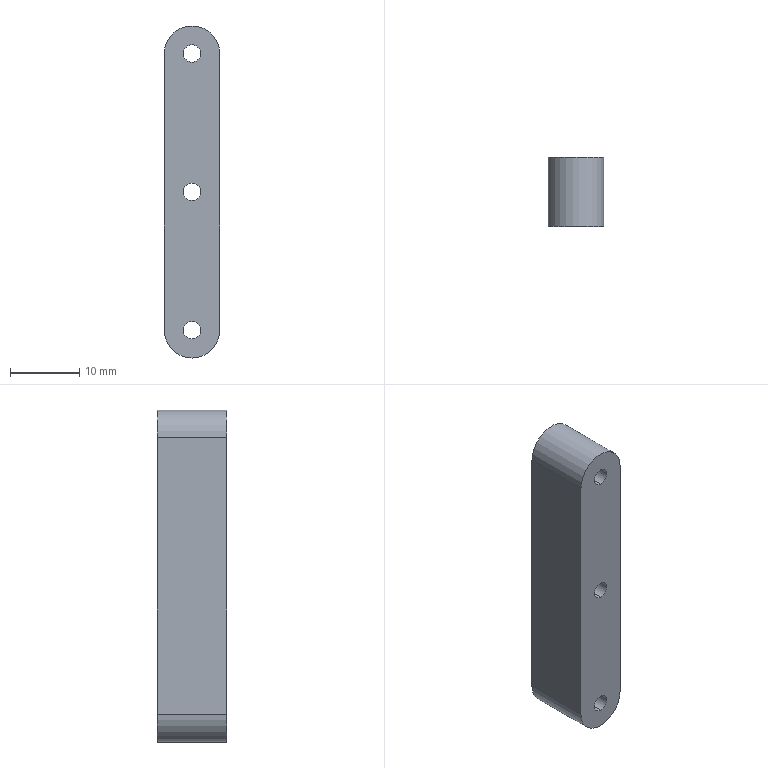Part | STEP file | 0246_209_Block | 1 solid | 13 faces | box 8 x 10 x 48 mm | volume 3555 mm3 | cylinder 9 | plane 4 | commonest cylinder face diameters 2.5 x6 8 x3
STEP:
#1=CARTESIAN_POINT('',(0.,0.,0.));
#2=DIRECTION('',(0.,0.,1.));
#3=DIRECTION('',(1.,0.,0.));
#4=AXIS2_PLACEMENT_3D('',#1,#2,#3);
#5=CARTESIAN_POINT('',(0.,0.,1.25));
#6=VERTEX_POINT('',#5);
#7=CARTESIAN_POINT('',(0.,10.,1.25));
#8=VERTEX_POINT('',#7);
#9=CARTESIAN_POINT('',(0.,10.,1.25));
#10=DIRECTION('',(0.,1.,0.));
#11=VECTOR('',#10,1.);
#12=LINE('',#9,#11);
#13=CARTESIAN_POINT('',(0.,10.,0.));
#14=DIRECTION('',(0.,1.,0.));
#15=DIRECTION('',(0.,0.,1.));
#16=AXIS2_PLACEMENT_3D('',#13,#14,#15);
#17=CYLINDRICAL_SURFACE('',#16,1.25);
#18=CARTESIAN_POINT('',(6.283,0.));
#19=DIRECTION('',(0.,1.));
#20=VECTOR('',#19,1.);
#21=LINE('',#18,#20);
#22=(GEOMETRIC_REPRESENTATION_CONTEXT(2)PARAMETRIC_REPRESENTATION_CONTEXT()REPRESENTATION_CONTEXT('',''));
#23=DEFINITIONAL_REPRESENTATION('',(#21),#22);
#24=PCURVE('',#17,#23);
#25=CARTESIAN_POINT('',(0.,10.,0.));
#26=DIRECTION('',(0.,1.,0.));
#27=DIRECTION('',(0.,0.,1.));
#28=AXIS2_PLACEMENT_3D('',#25,#26,#27);
#29=CYLINDRICAL_SURFACE('',#28,1.25);
#30=CARTESIAN_POINT('',(0.,0.));
#31=DIRECTION('',(0.,1.));
#32=VECTOR('',#31,1.);
#33=LINE('',#30,#32);
#34=(GEOMETRIC_REPRESENTATION_CONTEXT(2)PARAMETRIC_REPRESENTATION_CONTEXT()REPRESENTATION_CONTEXT('',''));
#35=DEFINITIONAL_REPRESENTATION('',(#33),#34);
#36=PCURVE('',#29,#35);
#37=SURFACE_CURVE('',#12,(#24,#36),.PCURVE_S1.);
#38=EDGE_CURVE('',#6,#8,#37,.T.);
#39=ORIENTED_EDGE('',*,*,#38,.T.);
#40=CARTESIAN_POINT('',(0.,10.,-1.25));
#41=VERTEX_POINT('',#40);
#42=CARTESIAN_POINT('',(0.,10.,0.));
#43=DIRECTION('',(0.,1.,0.));
#44=DIRECTION('',(0.,0.,1.));
#45=AXIS2_PLACEMENT_3D('',#42,#43,#44);
#46=CIRCLE('',#45,1.25);
#47=CARTESIAN_POINT('',(0.,0.));
#48=DIRECTION('',(1.,0.));
#49=VECTOR('',#48,1.);
#50=LINE('',#47,#49);
#51=(GEOMETRIC_REPRESENTATION_CONTEXT(2)PARAMETRIC_REPRESENTATION_CONTEXT()REPRESENTATION_CONTEXT('',''));
#52=DEFINITIONAL_REPRESENTATION('',(#50),#51);
#53=PCURVE('',#17,#52);
#54=CARTESIAN_POINT('',(0.,10.,0.));
#55=DIRECTION('',(0.,1.,0.));
#56=DIRECTION('',(0.,0.,1.));
#57=AXIS2_PLACEMENT_3D('',#54,#55,#56);
#58=PLANE('',#57);
#59=CARTESIAN_POINT('',(0.,0.));
#60=DIRECTION('',(1.,0.));
#61=AXIS2_PLACEMENT_2D('',#59,#60);
#62=CIRCLE('',#61,1.25);
#63=(GEOMETRIC_REPRESENTATION_CONTEXT(2)PARAMETRIC_REPRESENTATION_CONTEXT()REPRESENTATION_CONTEXT('',''));
#64=DEFINITIONAL_REPRESENTATION('',(#62),#63);
#65=PCURVE('',#58,#64);
#66=SURFACE_CURVE('',#46,(#53,#65),.PCURVE_S1.);
#67=EDGE_CURVE('',#41,#8,#66,.T.);
#68=ORIENTED_EDGE('',*,*,#67,.F.);
#69=CARTESIAN_POINT('',(0.,0.,-1.25));
#70=VERTEX_POINT('',#69);
#71=CARTESIAN_POINT('',(0.,10.,-1.25));
#72=DIRECTION('',(0.,1.,0.));
#73=VECTOR('',#72,1.);
#74=LINE('',#71,#73);
#75=CARTESIAN_POINT('',(3.142,0.));
#76=DIRECTION('',(0.,1.));
#77=VECTOR('',#76,1.);
#78=LINE('',#75,#77);
#79=(GEOMETRIC_REPRESENTATION_CONTEXT(2)PARAMETRIC_REPRESENTATION_CONTEXT()REPRESENTATION_CONTEXT('',''));
#80=DEFINITIONAL_REPRESENTATION('',(#78),#79);
#81=PCURVE('',#17,#80);
#82=CARTESIAN_POINT('',(3.142,0.));
#83=DIRECTION('',(0.,1.));
#84=VECTOR('',#83,1.);
#85=LINE('',#82,#84);
#86=(GEOMETRIC_REPRESENTATION_CONTEXT(2)PARAMETRIC_REPRESENTATION_CONTEXT()REPRESENTATION_CONTEXT('',''));
#87=DEFINITIONAL_REPRESENTATION('',(#85),#86);
#88=PCURVE('',#29,#87);
#89=SURFACE_CURVE('',#74,(#81,#88),.PCURVE_S1.);
#90=EDGE_CURVE('',#70,#41,#89,.T.);
#91=ORIENTED_EDGE('',*,*,#90,.F.);
#92=CARTESIAN_POINT('',(0.,0.,0.));
#93=DIRECTION('',(0.,1.,0.));
#94=DIRECTION('',(0.,0.,1.));
#95=AXIS2_PLACEMENT_3D('',#92,#93,#94);
#96=CIRCLE('',#95,1.25);
#97=CARTESIAN_POINT('',(0.,-10.));
#98=DIRECTION('',(1.,0.));
#99=VECTOR('',#98,1.);
#100=LINE('',#97,#99);
#101=(GEOMETRIC_REPRESENTATION_CONTEXT(2)PARAMETRIC_REPRESENTATION_CONTEXT()REPRESENTATION_CONTEXT('',''));
#102=DEFINITIONAL_REPRESENTATION('',(#100),#101);
#103=PCURVE('',#17,#102);
#104=CARTESIAN_POINT('',(0.,0.,0.));
#105=DIRECTION('',(0.,1.,0.));
#106=DIRECTION('',(0.,0.,1.));
#107=AXIS2_PLACEMENT_3D('',#104,#105,#106);
#108=PLANE('',#107);
#109=CARTESIAN_POINT('',(0.,0.));
#110=DIRECTION('',(1.,0.));
#111=AXIS2_PLACEMENT_2D('',#109,#110);
#112=CIRCLE('',#111,1.25);
#113=(GEOMETRIC_REPRESENTATION_CONTEXT(2)PARAMETRIC_REPRESENTATION_CONTEXT()REPRESENTATION_CONTEXT('',''));
#114=DEFINITIONAL_REPRESENTATION('',(#112),#113);
#115=PCURVE('',#108,#114);
#116=SURFACE_CURVE('',#96,(#103,#115),.PCURVE_S1.);
#117=EDGE_CURVE('',#70,#6,#116,.T.);
#118=ORIENTED_EDGE('',*,*,#117,.T.);
#119=EDGE_LOOP('',(#39,#68,#91,#118));
#120=FACE_BOUND('',#119,.F.);
#121=ADVANCED_FACE('',(#120),#17,.F.);
#122=CARTESIAN_POINT('',(0.,0.,-18.75));
#123=VERTEX_POINT('',#122);
#124=CARTESIAN_POINT('',(0.,10.,-18.75));
#125=VERTEX_POINT('',#124);
#126=CARTESIAN_POINT('',(0.,10.,-18.75));
#127=DIRECTION('',(0.,1.,0.));
#128=VECTOR('',#127,1.);
#129=LINE('',#126,#128);
#130=CARTESIAN_POINT('',(0.,10.,-20.));
#131=DIRECTION('',(0.,1.,0.));
#132=DIRECTION('',(0.,0.,1.));
#133=AXIS2_PLACEMENT_3D('',#130,#131,#132);
#134=CYLINDRICAL_SURFACE('',#133,1.25);
#135=CARTESIAN_POINT('',(6.283,0.));
#136=DIRECTION('',(0.,1.));
#137=VECTOR('',#136,1.);
#138=LINE('',#135,#137);
#139=(GEOMETRIC_REPRESENTATION_CONTEXT(2)PARAMETRIC_REPRESENTATION_CONTEXT()REPRESENTATION_CONTEXT('',''));
#140=DEFINITIONAL_REPRESENTATION('',(#138),#139);
#141=PCURVE('',#134,#140);
#142=CARTESIAN_POINT('',(0.,10.,-20.));
#143=DIRECTION('',(0.,1.,0.));
#144=DIRECTION('',(0.,0.,1.));
#145=AXIS2_PLACEMENT_3D('',#142,#143,#144);
#146=CYLINDRICAL_SURFACE('',#145,1.25);
#147=CARTESIAN_POINT('',(0.,0.));
#148=DIRECTION('',(0.,1.));
#149=VECTOR('',#148,1.);
#150=LINE('',#147,#149);
#151=(GEOMETRIC_REPRESENTATION_CONTEXT(2)PARAMETRIC_REPRESENTATION_CONTEXT()REPRESENTATION_CONTEXT('',''));
#152=DEFINITIONAL_REPRESENTATION('',(#150),#151);
#153=PCURVE('',#146,#152);
#154=SURFACE_CURVE('',#129,(#141,#153),.PCURVE_S1.);
#155=EDGE_CURVE('',#123,#125,#154,.T.);
#156=ORIENTED_EDGE('',*,*,#155,.T.);
#157=CARTESIAN_POINT('',(0.,10.,-21.25));
#158=VERTEX_POINT('',#157);
#159=CARTESIAN_POINT('',(0.,10.,-20.));
#160=DIRECTION('',(0.,1.,0.));
#161=DIRECTION('',(0.,0.,1.));
#162=AXIS2_PLACEMENT_3D('',#159,#160,#161);
#163=CIRCLE('',#162,1.25);
#164=CARTESIAN_POINT('',(0.,0.));
#165=DIRECTION('',(1.,0.));
#166=VECTOR('',#165,1.);
#167=LINE('',#164,#166);
#168=(GEOMETRIC_REPRESENTATION_CONTEXT(2)PARAMETRIC_REPRESENTATION_CONTEXT()REPRESENTATION_CONTEXT('',''));
#169=DEFINITIONAL_REPRESENTATION('',(#167),#168);
#170=PCURVE('',#134,#169);
#171=CARTESIAN_POINT('',(-20.,0.));
#172=DIRECTION('',(1.,0.));
#173=AXIS2_PLACEMENT_2D('',#171,#172);
#174=CIRCLE('',#173,1.25);
#175=(GEOMETRIC_REPRESENTATION_CONTEXT(2)PARAMETRIC_REPRESENTATION_CONTEXT()REPRESENTATION_CONTEXT('',''));
#176=DEFINITIONAL_REPRESENTATION('',(#174),#175);
#177=PCURVE('',#58,#176);
#178=SURFACE_CURVE('',#163,(#170,#177),.PCURVE_S1.);
#179=EDGE_CURVE('',#158,#125,#178,.T.);
#180=ORIENTED_EDGE('',*,*,#179,.F.);
#181=CARTESIAN_POINT('',(0.,0.,-21.25));
#182=VERTEX_POINT('',#181);
#183=CARTESIAN_POINT('',(0.,10.,-21.25));
#184=DIRECTION('',(0.,1.,0.));
#185=VECTOR('',#184,1.);
#186=LINE('',#183,#185);
#187=CARTESIAN_POINT('',(3.142,0.));
#188=DIRECTION('',(0.,1.));
#189=VECTOR('',#188,1.);
#190=LINE('',#187,#189);
#191=(GEOMETRIC_REPRESENTATION_CONTEXT(2)PARAMETRIC_REPRESENTATION_CONTEXT()REPRESENTATION_CONTEXT('',''));
#192=DEFINITIONAL_REPRESENTATION('',(#190),#191);
#193=PCURVE('',#134,#192);
#194=CARTESIAN_POINT('',(3.142,0.));
#195=DIRECTION('',(0.,1.));
#196=VECTOR('',#195,1.);
#197=LINE('',#194,#196);
#198=(GEOMETRIC_REPRESENTATION_CONTEXT(2)PARAMETRIC_REPRESENTATION_CONTEXT()REPRESENTATION_CONTEXT('',''));
#199=DEFINITIONAL_REPRESENTATION('',(#197),#198);
#200=PCURVE('',#146,#199);
#201=SURFACE_CURVE('',#186,(#193,#200),.PCURVE_S1.);
#202=EDGE_CURVE('',#182,#158,#201,.T.);
#203=ORIENTED_EDGE('',*,*,#202,.F.);
#204=CARTESIAN_POINT('',(0.,0.,-20.));
#205=DIRECTION('',(0.,1.,0.));
#206=DIRECTION('',(0.,0.,1.));
#207=AXIS2_PLACEMENT_3D('',#204,#205,#206);
#208=CIRCLE('',#207,1.25);
#209=CARTESIAN_POINT('',(0.,-10.));
#210=DIRECTION('',(1.,0.));
#211=VECTOR('',#210,1.);
#212=LINE('',#209,#211);
#213=(GEOMETRIC_REPRESENTATION_CONTEXT(2)PARAMETRIC_REPRESENTATION_CONTEXT()REPRESENTATION_CONTEXT('',''));
#214=DEFINITIONAL_REPRESENTATION('',(#212),#213);
#215=PCURVE('',#134,#214);
#216=CARTESIAN_POINT('',(-20.,0.));
#217=DIRECTION('',(1.,0.));
#218=AXIS2_PLACEMENT_2D('',#216,#217);
#219=CIRCLE('',#218,1.25);
#220=(GEOMETRIC_REPRESENTATION_CONTEXT(2)PARAMETRIC_REPRESENTATION_CONTEXT()REPRESENTATION_CONTEXT('',''));
#221=DEFINITIONAL_REPRESENTATION('',(#219),#220);
#222=PCURVE('',#108,#221);
#223=SURFACE_CURVE('',#208,(#215,#222),.PCURVE_S1.);
#224=EDGE_CURVE('',#182,#123,#223,.T.);
#225=ORIENTED_EDGE('',*,*,#224,.T.);
#226=EDGE_LOOP('',(#156,#180,#203,#225));
#227=FACE_BOUND('',#226,.F.);
#228=ADVANCED_FACE('',(#227),#134,.F.);
#229=CARTESIAN_POINT('',(0.,0.,-38.75));
#230=VERTEX_POINT('',#229);
#231=CARTESIAN_POINT('',(0.,10.,-38.75));
#232=VERTEX_POINT('',#231);
#233=CARTESIAN_POINT('',(0.,10.,-38.75));
#234=DIRECTION('',(0.,1.,0.));
#235=VECTOR('',#234,1.);
#236=LINE('',#233,#235);
#237=CARTESIAN_POINT('',(0.,10.,-40.));
#238=DIRECTION('',(0.,1.,0.));
#239=DIRECTION('',(0.,0.,1.));
#240=AXIS2_PLACEMENT_3D('',#237,#238,#239);
#241=CYLINDRICAL_SURFACE('',#240,1.25);
#242=CARTESIAN_POINT('',(6.283,0.));
#243=DIRECTION('',(0.,1.));
#244=VECTOR('',#243,1.);
#245=LINE('',#242,#244);
#246=(GEOMETRIC_REPRESENTATION_CONTEXT(2)PARAMETRIC_REPRESENTATION_CONTEXT()REPRESENTATION_CONTEXT('',''));
#247=DEFINITIONAL_REPRESENTATION('',(#245),#246);
#248=PCURVE('',#241,#247);
#249=CARTESIAN_POINT('',(0.,10.,-40.));
#250=DIRECTION('',(0.,1.,0.));
#251=DIRECTION('',(0.,0.,1.));
#252=AXIS2_PLACEMENT_3D('',#249,#250,#251);
#253=CYLINDRICAL_SURFACE('',#252,1.25);
#254=CARTESIAN_POINT('',(0.,0.));
#255=DIRECTION('',(0.,1.));
#256=VECTOR('',#255,1.);
#257=LINE('',#254,#256);
#258=(GEOMETRIC_REPRESENTATION_CONTEXT(2)PARAMETRIC_REPRESENTATION_CONTEXT()REPRESENTATION_CONTEXT('',''));
#259=DEFINITIONAL_REPRESENTATION('',(#257),#258);
#260=PCURVE('',#253,#259);
#261=SURFACE_CURVE('',#236,(#248,#260),.PCURVE_S1.);
#262=EDGE_CURVE('',#230,#232,#261,.T.);
#263=ORIENTED_EDGE('',*,*,#262,.T.);
#264=CARTESIAN_POINT('',(0.,10.,-41.25));
#265=VERTEX_POINT('',#264);
#266=CARTESIAN_POINT('',(0.,10.,-40.));
#267=DIRECTION('',(0.,1.,0.));
#268=DIRECTION('',(0.,0.,1.));
#269=AXIS2_PLACEMENT_3D('',#266,#267,#268);
#270=CIRCLE('',#269,1.25);
#271=CARTESIAN_POINT('',(0.,0.));
#272=DIRECTION('',(1.,0.));
#273=VECTOR('',#272,1.);
#274=LINE('',#271,#273);
#275=(GEOMETRIC_REPRESENTATION_CONTEXT(2)PARAMETRIC_REPRESENTATION_CONTEXT()REPRESENTATION_CONTEXT('',''));
#276=DEFINITIONAL_REPRESENTATION('',(#274),#275);
#277=PCURVE('',#241,#276);
#278=CARTESIAN_POINT('',(-40.,0.));
#279=DIRECTION('',(1.,0.));
#280=AXIS2_PLACEMENT_2D('',#278,#279);
#281=CIRCLE('',#280,1.25);
#282=(GEOMETRIC_REPRESENTATION_CONTEXT(2)PARAMETRIC_REPRESENTATION_CONTEXT()REPRESENTATION_CONTEXT('',''));
#283=DEFINITIONAL_REPRESENTATION('',(#281),#282);
#284=PCURVE('',#58,#283);
#285=SURFACE_CURVE('',#270,(#277,#284),.PCURVE_S1.);
#286=EDGE_CURVE('',#265,#232,#285,.T.);
#287=ORIENTED_EDGE('',*,*,#286,.F.);
#288=CARTESIAN_POINT('',(0.,0.,-41.25));
#289=VERTEX_POINT('',#288);
#290=CARTESIAN_POINT('',(0.,10.,-41.25));
#291=DIRECTION('',(0.,1.,0.));
#292=VECTOR('',#291,1.);
#293=LINE('',#290,#292);
#294=CARTESIAN_POINT('',(3.142,0.));
#295=DIRECTION('',(0.,1.));
#296=VECTOR('',#295,1.);
#297=LINE('',#294,#296);
#298=(GEOMETRIC_REPRESENTATION_CONTEXT(2)PARAMETRIC_REPRESENTATION_CONTEXT()REPRESENTATION_CONTEXT('',''));
#299=DEFINITIONAL_REPRESENTATION('',(#297),#298);
#300=PCURVE('',#241,#299);
#301=CARTESIAN_POINT('',(3.142,0.));
#302=DIRECTION('',(0.,1.));
#303=VECTOR('',#302,1.);
#304=LINE('',#301,#303);
#305=(GEOMETRIC_REPRESENTATION_CONTEXT(2)PARAMETRIC_REPRESENTATION_CONTEXT()REPRESENTATION_CONTEXT('',''));
#306=DEFINITIONAL_REPRESENTATION('',(#304),#305);
#307=PCURVE('',#253,#306);
#308=SURFACE_CURVE('',#293,(#300,#307),.PCURVE_S1.);
#309=EDGE_CURVE('',#289,#265,#308,.T.);
#310=ORIENTED_EDGE('',*,*,#309,.F.);
#311=CARTESIAN_POINT('',(0.,0.,-40.));
#312=DIRECTION('',(0.,1.,0.));
#313=DIRECTION('',(0.,0.,1.));
#314=AXIS2_PLACEMENT_3D('',#311,#312,#313);
#315=CIRCLE('',#314,1.25);
#316=CARTESIAN_POINT('',(0.,-10.));
#317=DIRECTION('',(1.,0.));
#318=VECTOR('',#317,1.);
#319=LINE('',#316,#318);
#320=(GEOMETRIC_REPRESENTATION_CONTEXT(2)PARAMETRIC_REPRESENTATION_CONTEXT()REPRESENTATION_CONTEXT('',''));
#321=DEFINITIONAL_REPRESENTATION('',(#319),#320);
#322=PCURVE('',#241,#321);
#323=CARTESIAN_POINT('',(-40.,0.));
#324=DIRECTION('',(1.,0.));
#325=AXIS2_PLACEMENT_2D('',#323,#324);
#326=CIRCLE('',#325,1.25);
#327=(GEOMETRIC_REPRESENTATION_CONTEXT(2)PARAMETRIC_REPRESENTATION_CONTEXT()REPRESENTATION_CONTEXT('',''));
#328=DEFINITIONAL_REPRESENTATION('',(#326),#327);
#329=PCURVE('',#108,#328);
#330=SURFACE_CURVE('',#315,(#322,#329),.PCURVE_S1.);
#331=EDGE_CURVE('',#289,#230,#330,.T.);
#332=ORIENTED_EDGE('',*,*,#331,.T.);
#333=EDGE_LOOP('',(#263,#287,#310,#332));
#334=FACE_BOUND('',#333,.F.);
#335=ADVANCED_FACE('',(#334),#241,.F.);
#336=CARTESIAN_POINT('',(0.,10.,-44.));
#337=VERTEX_POINT('',#336);
#338=CARTESIAN_POINT('',(-4.,10.,-40.));
#339=VERTEX_POINT('',#338);
#340=CARTESIAN_POINT('',(0.,10.,-40.));
#341=DIRECTION('',(0.,1.,0.));
#342=DIRECTION('',(0.,0.,1.));
#343=AXIS2_PLACEMENT_3D('',#340,#341,#342);
#344=CIRCLE('',#343,4.);
#345=CARTESIAN_POINT('',(0.,10.,-40.));
#346=DIRECTION('',(0.,-1.,0.));
#347=DIRECTION('',(0.,0.,-1.));
#348=AXIS2_PLACEMENT_3D('',#345,#346,#347);
#349=CYLINDRICAL_SURFACE('',#348,4.);
#350=CARTESIAN_POINT('',(9.425,0.));
#351=DIRECTION('',(-1.,0.));
#352=VECTOR('',#351,1.);
#353=LINE('',#350,#352);
#354=(GEOMETRIC_REPRESENTATION_CONTEXT(2)PARAMETRIC_REPRESENTATION_CONTEXT()REPRESENTATION_CONTEXT('',''));
#355=DEFINITIONAL_REPRESENTATION('',(#353),#354);
#356=PCURVE('',#349,#355);
#357=CARTESIAN_POINT('',(-40.,0.));
#358=DIRECTION('',(1.,0.));
#359=AXIS2_PLACEMENT_2D('',#357,#358);
#360=CIRCLE('',#359,4.);
#361=(GEOMETRIC_REPRESENTATION_CONTEXT(2)PARAMETRIC_REPRESENTATION_CONTEXT()REPRESENTATION_CONTEXT('',''));
#362=DEFINITIONAL_REPRESENTATION('',(#360),#361);
#363=PCURVE('',#58,#362);
#364=SURFACE_CURVE('',#344,(#356,#363),.PCURVE_S1.);
#365=EDGE_CURVE('',#337,#339,#364,.T.);
#366=ORIENTED_EDGE('',*,*,#365,.F.);
#367=CARTESIAN_POINT('',(0.,0.,-44.));
#368=VERTEX_POINT('',#367);
#369=CARTESIAN_POINT('',(0.,10.,-44.));
#370=DIRECTION('',(0.,-1.,0.));
#371=VECTOR('',#370,1.);
#372=LINE('',#369,#371);
#373=CARTESIAN_POINT('',(6.283,0.));
#374=DIRECTION('',(0.,1.));
#375=VECTOR('',#374,1.);
#376=LINE('',#373,#375);
#377=(GEOMETRIC_REPRESENTATION_CONTEXT(2)PARAMETRIC_REPRESENTATION_CONTEXT()REPRESENTATION_CONTEXT('',''));
#378=DEFINITIONAL_REPRESENTATION('',(#376),#377);
#379=PCURVE('',#349,#378);
#380=CARTESIAN_POINT('',(0.,10.,-40.));
#381=DIRECTION('',(0.,-1.,0.));
#382=DIRECTION('',(0.,0.,-1.));
#383=AXIS2_PLACEMENT_3D('',#380,#381,#382);
#384=CYLINDRICAL_SURFACE('',#383,4.);
#385=CARTESIAN_POINT('',(0.,0.));
#386=DIRECTION('',(0.,1.));
#387=VECTOR('',#386,1.);
#388=LINE('',#385,#387);
#389=(GEOMETRIC_REPRESENTATION_CONTEXT(2)PARAMETRIC_REPRESENTATION_CONTEXT()REPRESENTATION_CONTEXT('',''));
#390=DEFINITIONAL_REPRESENTATION('',(#388),#389);
#391=PCURVE('',#384,#390);
#392=SURFACE_CURVE('',#372,(#379,#391),.PCURVE_S1.);
#393=EDGE_CURVE('',#337,#368,#392,.T.);
#394=ORIENTED_EDGE('',*,*,#393,.T.);
#395=CARTESIAN_POINT('',(-4.,0.,-40.));
#396=VERTEX_POINT('',#395);
#397=CARTESIAN_POINT('',(0.,0.,-40.));
#398=DIRECTION('',(0.,1.,0.));
#399=DIRECTION('',(0.,0.,1.));
#400=AXIS2_PLACEMENT_3D('',#397,#398,#399);
#401=CIRCLE('',#400,4.);
#402=CARTESIAN_POINT('',(9.425,10.));
#403=DIRECTION('',(-1.,0.));
#404=VECTOR('',#403,1.);
#405=LINE('',#402,#404);
#406=(GEOMETRIC_REPRESENTATION_CONTEXT(2)PARAMETRIC_REPRESENTATION_CONTEXT()REPRESENTATION_CONTEXT('',''));
#407=DEFINITIONAL_REPRESENTATION('',(#405),#406);
#408=PCURVE('',#349,#407);
#409=CARTESIAN_POINT('',(-40.,0.));
#410=DIRECTION('',(1.,0.));
#411=AXIS2_PLACEMENT_2D('',#409,#410);
#412=CIRCLE('',#411,4.);
#413=(GEOMETRIC_REPRESENTATION_CONTEXT(2)PARAMETRIC_REPRESENTATION_CONTEXT()REPRESENTATION_CONTEXT('',''));
#414=DEFINITIONAL_REPRESENTATION('',(#412),#413);
#415=PCURVE('',#108,#414);
#416=SURFACE_CURVE('',#401,(#408,#415),.PCURVE_S1.);
#417=EDGE_CURVE('',#368,#396,#416,.T.);
#418=ORIENTED_EDGE('',*,*,#417,.T.);
#419=CARTESIAN_POINT('',(-4.,10.,-40.));
#420=DIRECTION('',(0.,-1.,0.));
#421=VECTOR('',#420,1.);
#422=LINE('',#419,#421);
#423=CARTESIAN_POINT('',(4.712,0.));
#424=DIRECTION('',(0.,1.));
#425=VECTOR('',#424,1.);
#426=LINE('',#423,#425);
#427=(GEOMETRIC_REPRESENTATION_CONTEXT(2)PARAMETRIC_REPRESENTATION_CONTEXT()REPRESENTATION_CONTEXT('',''));
#428=DEFINITIONAL_REPRESENTATION('',(#426),#427);
#429=PCURVE('',#349,#428);
#430=CARTESIAN_POINT('',(-4.,10.,0.));
#431=DIRECTION('',(1.,0.,0.));
#432=DIRECTION('',(0.,0.,-1.));
#433=AXIS2_PLACEMENT_3D('',#430,#431,#432);
#434=PLANE('',#433);
#435=CARTESIAN_POINT('',(40.,0.));
#436=DIRECTION('',(0.,-1.));
#437=VECTOR('',#436,1.);
#438=LINE('',#435,#437);
#439=(GEOMETRIC_REPRESENTATION_CONTEXT(2)PARAMETRIC_REPRESENTATION_CONTEXT()REPRESENTATION_CONTEXT('',''));
#440=DEFINITIONAL_REPRESENTATION('',(#438),#439);
#441=PCURVE('',#434,#440);
#442=SURFACE_CURVE('',#422,(#429,#441),.PCURVE_S1.);
#443=EDGE_CURVE('',#339,#396,#442,.T.);
#444=ORIENTED_EDGE('',*,*,#443,.F.);
#445=EDGE_LOOP('',(#366,#394,#418,#444));
#446=FACE_BOUND('',#445,.T.);
#447=ADVANCED_FACE('',(#446),#349,.T.);
#448=CARTESIAN_POINT('',(-4.,0.,0.));
#449=VERTEX_POINT('',#448);
#450=CARTESIAN_POINT('',(4.,0.,0.));
#451=VERTEX_POINT('',#450);
#452=CARTESIAN_POINT('',(0.,0.,0.));
#453=DIRECTION('',(0.,1.,0.));
#454=DIRECTION('',(0.,0.,1.));
#455=AXIS2_PLACEMENT_3D('',#452,#453,#454);
#456=CIRCLE('',#455,4.);
#457=CARTESIAN_POINT('',(0.,10.,0.));
#458=DIRECTION('',(0.,-1.,0.));
#459=DIRECTION('',(0.,0.,-1.));
#460=AXIS2_PLACEMENT_3D('',#457,#458,#459);
#461=CYLINDRICAL_SURFACE('',#460,4.);
#462=CARTESIAN_POINT('',(9.425,10.));
#463=DIRECTION('',(-1.,0.));
#464=VECTOR('',#463,1.);
#465=LINE('',#462,#464);
#466=(GEOMETRIC_REPRESENTATION_CONTEXT(2)PARAMETRIC_REPRESENTATION_CONTEXT()REPRESENTATION_CONTEXT('',''));
#467=DEFINITIONAL_REPRESENTATION('',(#465),#466);
#468=PCURVE('',#461,#467);
#469=CARTESIAN_POINT('',(0.,0.));
#470=DIRECTION('',(1.,0.));
#471=AXIS2_PLACEMENT_2D('',#469,#470);
#472=CIRCLE('',#471,4.);
#473=(GEOMETRIC_REPRESENTATION_CONTEXT(2)PARAMETRIC_REPRESENTATION_CONTEXT()REPRESENTATION_CONTEXT('',''));
#474=DEFINITIONAL_REPRESENTATION('',(#472),#473);
#475=PCURVE('',#108,#474);
#476=SURFACE_CURVE('',#456,(#468,#475),.PCURVE_S1.);
#477=EDGE_CURVE('',#449,#451,#476,.T.);
#478=ORIENTED_EDGE('',*,*,#477,.T.);
#479=CARTESIAN_POINT('',(4.,10.,0.));
#480=VERTEX_POINT('',#479);
#481=CARTESIAN_POINT('',(4.,10.,0.));
#482=DIRECTION('',(0.,-1.,0.));
#483=VECTOR('',#482,1.);
#484=LINE('',#481,#483);
#485=CARTESIAN_POINT('',(1.571,0.));
#486=DIRECTION('',(0.,1.));
#487=VECTOR('',#486,1.);
#488=LINE('',#485,#487);
#489=(GEOMETRIC_REPRESENTATION_CONTEXT(2)PARAMETRIC_REPRESENTATION_CONTEXT()REPRESENTATION_CONTEXT('',''));
#490=DEFINITIONAL_REPRESENTATION('',(#488),#489);
#491=PCURVE('',#461,#490);
#492=CARTESIAN_POINT('',(4.,10.,0.));
#493=DIRECTION('',(-1.,0.,0.));
#494=DIRECTION('',(0.,0.,1.));
#495=AXIS2_PLACEMENT_3D('',#492,#493,#494);
#496=PLANE('',#495);
#497=CARTESIAN_POINT('',(0.,0.));
#498=DIRECTION('',(0.,-1.));
#499=VECTOR('',#498,1.);
#500=LINE('',#497,#499);
#501=(GEOMETRIC_REPRESENTATION_CONTEXT(2)PARAMETRIC_REPRESENTATION_CONTEXT()REPRESENTATION_CONTEXT('',''));
#502=DEFINITIONAL_REPRESENTATION('',(#500),#501);
#503=PCURVE('',#496,#502);
#504=SURFACE_CURVE('',#484,(#491,#503),.PCURVE_S1.);
#505=EDGE_CURVE('',#480,#451,#504,.T.);
#506=ORIENTED_EDGE('',*,*,#505,.F.);
#507=CARTESIAN_POINT('',(-4.,10.,0.));
#508=VERTEX_POINT('',#507);
#509=CARTESIAN_POINT('',(0.,10.,0.));
#510=DIRECTION('',(0.,1.,0.));
#511=DIRECTION('',(0.,0.,1.));
#512=AXIS2_PLACEMENT_3D('',#509,#510,#511);
#513=CIRCLE('',#512,4.);
#514=CARTESIAN_POINT('',(9.425,0.));
#515=DIRECTION('',(-1.,0.));
#516=VECTOR('',#515,1.);
#517=LINE('',#514,#516);
#518=(GEOMETRIC_REPRESENTATION_CONTEXT(2)PARAMETRIC_REPRESENTATION_CONTEXT()REPRESENTATION_CONTEXT('',''));
#519=DEFINITIONAL_REPRESENTATION('',(#517),#518);
#520=PCURVE('',#461,#519);
#521=CARTESIAN_POINT('',(0.,0.));
#522=DIRECTION('',(1.,0.));
#523=AXIS2_PLACEMENT_2D('',#521,#522);
#524=CIRCLE('',#523,4.);
#525=(GEOMETRIC_REPRESENTATION_CONTEXT(2)PARAMETRIC_REPRESENTATION_CONTEXT()REPRESENTATION_CONTEXT('',''));
#526=DEFINITIONAL_REPRESENTATION('',(#524),#525);
#527=PCURVE('',#58,#526);
#528=SURFACE_CURVE('',#513,(#520,#527),.PCURVE_S1.);
#529=EDGE_CURVE('',#508,#480,#528,.T.);
#530=ORIENTED_EDGE('',*,*,#529,.F.);
#531=CARTESIAN_POINT('',(-4.,10.,0.));
#532=DIRECTION('',(0.,-1.,0.));
#533=VECTOR('',#532,1.);
#534=LINE('',#531,#533);
#535=CARTESIAN_POINT('',(4.712,0.));
#536=DIRECTION('',(0.,1.));
#537=VECTOR('',#536,1.);
#538=LINE('',#535,#537);
#539=(GEOMETRIC_REPRESENTATION_CONTEXT(2)PARAMETRIC_REPRESENTATION_CONTEXT()REPRESENTATION_CONTEXT('',''));
#540=DEFINITIONAL_REPRESENTATION('',(#538),#539);
#541=PCURVE('',#461,#540);
#542=CARTESIAN_POINT('',(0.,0.));
#543=DIRECTION('',(0.,-1.));
#544=VECTOR('',#543,1.);
#545=LINE('',#542,#544);
#546=(GEOMETRIC_REPRESENTATION_CONTEXT(2)PARAMETRIC_REPRESENTATION_CONTEXT()REPRESENTATION_CONTEXT('',''));
#547=DEFINITIONAL_REPRESENTATION('',(#545),#546);
#548=PCURVE('',#434,#547);
#549=SURFACE_CURVE('',#534,(#541,#548),.PCURVE_S1.);
#550=EDGE_CURVE('',#508,#449,#549,.T.);
#551=ORIENTED_EDGE('',*,*,#550,.T.);
#552=EDGE_LOOP('',(#478,#506,#530,#551));
#553=FACE_BOUND('',#552,.T.);
#554=ADVANCED_FACE('',(#553),#461,.T.);
#555=CARTESIAN_POINT('',(4.,0.,-40.));
#556=VERTEX_POINT('',#555);
#557=CARTESIAN_POINT('',(4.,0.,0.));
#558=DIRECTION('',(0.,0.,-1.));
#559=VECTOR('',#558,1.);
#560=LINE('',#557,#559);
#561=CARTESIAN_POINT('',(0.,-10.));
#562=DIRECTION('',(-1.,0.));
#563=VECTOR('',#562,1.);
#564=LINE('',#561,#563);
#565=(GEOMETRIC_REPRESENTATION_CONTEXT(2)PARAMETRIC_REPRESENTATION_CONTEXT()REPRESENTATION_CONTEXT('',''));
#566=DEFINITIONAL_REPRESENTATION('',(#564),#565);
#567=PCURVE('',#496,#566);
#568=CARTESIAN_POINT('',(0.,4.));
#569=DIRECTION('',(-1.,0.));
#570=VECTOR('',#569,1.);
#571=LINE('',#568,#570);
#572=(GEOMETRIC_REPRESENTATION_CONTEXT(2)PARAMETRIC_REPRESENTATION_CONTEXT()REPRESENTATION_CONTEXT('',''));
#573=DEFINITIONAL_REPRESENTATION('',(#571),#572);
#574=PCURVE('',#108,#573);
#575=SURFACE_CURVE('',#560,(#567,#574),.PCURVE_S1.);
#576=EDGE_CURVE('',#451,#556,#575,.T.);
#577=ORIENTED_EDGE('',*,*,#576,.T.);
#578=CARTESIAN_POINT('',(4.,10.,-40.));
#579=VERTEX_POINT('',#578);
#580=CARTESIAN_POINT('',(4.,10.,-40.));
#581=DIRECTION('',(0.,-1.,0.));
#582=VECTOR('',#581,1.);
#583=LINE('',#580,#582);
#584=CARTESIAN_POINT('',(-40.,0.));
#585=DIRECTION('',(0.,-1.));
#586=VECTOR('',#585,1.);
#587=LINE('',#584,#586);
#588=(GEOMETRIC_REPRESENTATION_CONTEXT(2)PARAMETRIC_REPRESENTATION_CONTEXT()REPRESENTATION_CONTEXT('',''));
#589=DEFINITIONAL_REPRESENTATION('',(#587),#588);
#590=PCURVE('',#496,#589);
#591=CARTESIAN_POINT('',(1.571,0.));
#592=DIRECTION('',(0.,1.));
#593=VECTOR('',#592,1.);
#594=LINE('',#591,#593);
#595=(GEOMETRIC_REPRESENTATION_CONTEXT(2)PARAMETRIC_REPRESENTATION_CONTEXT()REPRESENTATION_CONTEXT('',''));
#596=DEFINITIONAL_REPRESENTATION('',(#594),#595);
#597=PCURVE('',#384,#596);
#598=SURFACE_CURVE('',#583,(#590,#597),.PCURVE_S1.);
#599=EDGE_CURVE('',#579,#556,#598,.T.);
#600=ORIENTED_EDGE('',*,*,#599,.F.);
#601=CARTESIAN_POINT('',(4.,10.,0.));
#602=DIRECTION('',(0.,0.,-1.));
#603=VECTOR('',#602,1.);
#604=LINE('',#601,#603);
#605=CARTESIAN_POINT('',(0.,0.));
#606=DIRECTION('',(-1.,0.));
#607=VECTOR('',#606,1.);
#608=LINE('',#605,#607);
#609=(GEOMETRIC_REPRESENTATION_CONTEXT(2)PARAMETRIC_REPRESENTATION_CONTEXT()REPRESENTATION_CONTEXT('',''));
#610=DEFINITIONAL_REPRESENTATION('',(#608),#609);
#611=PCURVE('',#496,#610);
#612=CARTESIAN_POINT('',(0.,4.));
#613=DIRECTION('',(-1.,0.));
#614=VECTOR('',#613,1.);
#615=LINE('',#612,#614);
#616=(GEOMETRIC_REPRESENTATION_CONTEXT(2)PARAMETRIC_REPRESENTATION_CONTEXT()REPRESENTATION_CONTEXT('',''));
#617=DEFINITIONAL_REPRESENTATION('',(#615),#616);
#618=PCURVE('',#58,#617);
#619=SURFACE_CURVE('',#604,(#611,#618),.PCURVE_S1.);
#620=EDGE_CURVE('',#480,#579,#619,.T.);
#621=ORIENTED_EDGE('',*,*,#620,.F.);
#622=ORIENTED_EDGE('',*,*,#505,.T.);
#623=EDGE_LOOP('',(#577,#600,#621,#622));
#624=FACE_BOUND('',#623,.T.);
#625=ADVANCED_FACE('',(#624),#496,.F.);
#626=ORIENTED_EDGE('',*,*,#393,.F.);
#627=CARTESIAN_POINT('',(0.,10.,-40.));
#628=DIRECTION('',(0.,1.,0.));
#629=DIRECTION('',(0.,0.,1.));
#630=AXIS2_PLACEMENT_3D('',#627,#628,#629);
#631=CIRCLE('',#630,4.);
#632=CARTESIAN_POINT('',(3.142,0.));
#633=DIRECTION('',(-1.,0.));
#634=VECTOR('',#633,1.);
#635=LINE('',#632,#634);
#636=(GEOMETRIC_REPRESENTATION_CONTEXT(2)PARAMETRIC_REPRESENTATION_CONTEXT()REPRESENTATION_CONTEXT('',''));
#637=DEFINITIONAL_REPRESENTATION('',(#635),#636);
#638=PCURVE('',#384,#637);
#639=CARTESIAN_POINT('',(-40.,0.));
#640=DIRECTION('',(1.,0.));
#641=AXIS2_PLACEMENT_2D('',#639,#640);
#642=CIRCLE('',#641,4.);
#643=(GEOMETRIC_REPRESENTATION_CONTEXT(2)PARAMETRIC_REPRESENTATION_CONTEXT()REPRESENTATION_CONTEXT('',''));
#644=DEFINITIONAL_REPRESENTATION('',(#642),#643);
#645=PCURVE('',#58,#644);
#646=SURFACE_CURVE('',#631,(#638,#645),.PCURVE_S1.);
#647=EDGE_CURVE('',#579,#337,#646,.T.);
#648=ORIENTED_EDGE('',*,*,#647,.F.);
#649=ORIENTED_EDGE('',*,*,#599,.T.);
#650=CARTESIAN_POINT('',(0.,0.,-40.));
#651=DIRECTION('',(0.,1.,0.));
#652=DIRECTION('',(0.,0.,1.));
#653=AXIS2_PLACEMENT_3D('',#650,#651,#652);
#654=CIRCLE('',#653,4.);
#655=CARTESIAN_POINT('',(3.142,10.));
#656=DIRECTION('',(-1.,0.));
#657=VECTOR('',#656,1.);
#658=LINE('',#655,#657);
#659=(GEOMETRIC_REPRESENTATION_CONTEXT(2)PARAMETRIC_REPRESENTATION_CONTEXT()REPRESENTATION_CONTEXT('',''));
#660=DEFINITIONAL_REPRESENTATION('',(#658),#659);
#661=PCURVE('',#384,#660);
#662=CARTESIAN_POINT('',(-40.,0.));
#663=DIRECTION('',(1.,0.));
#664=AXIS2_PLACEMENT_2D('',#662,#663);
#665=CIRCLE('',#664,4.);
#666=(GEOMETRIC_REPRESENTATION_CONTEXT(2)PARAMETRIC_REPRESENTATION_CONTEXT()REPRESENTATION_CONTEXT('',''));
#667=DEFINITIONAL_REPRESENTATION('',(#665),#666);
#668=PCURVE('',#108,#667);
#669=SURFACE_CURVE('',#654,(#661,#668),.PCURVE_S1.);
#670=EDGE_CURVE('',#556,#368,#669,.T.);
#671=ORIENTED_EDGE('',*,*,#670,.T.);
#672=EDGE_LOOP('',(#626,#648,#649,#671));
#673=FACE_BOUND('',#672,.T.);
#674=ADVANCED_FACE('',(#673),#384,.T.);
#675=CARTESIAN_POINT('',(-4.,0.,0.));
#676=DIRECTION('',(0.,0.,1.));
#677=VECTOR('',#676,1.);
#678=LINE('',#675,#677);
#679=CARTESIAN_POINT('',(0.,-10.));
#680=DIRECTION('',(-1.,0.));
#681=VECTOR('',#680,1.);
#682=LINE('',#679,#681);
#683=(GEOMETRIC_REPRESENTATION_CONTEXT(2)PARAMETRIC_REPRESENTATION_CONTEXT()REPRESENTATION_CONTEXT('',''));
#684=DEFINITIONAL_REPRESENTATION('',(#682),#683);
#685=PCURVE('',#434,#684);
#686=CARTESIAN_POINT('',(0.,-4.));
#687=DIRECTION('',(1.,0.));
#688=VECTOR('',#687,1.);
#689=LINE('',#686,#688);
#690=(GEOMETRIC_REPRESENTATION_CONTEXT(2)PARAMETRIC_REPRESENTATION_CONTEXT()REPRESENTATION_CONTEXT('',''));
#691=DEFINITIONAL_REPRESENTATION('',(#689),#690);
#692=PCURVE('',#108,#691);
#693=SURFACE_CURVE('',#678,(#685,#692),.PCURVE_S1.);
#694=EDGE_CURVE('',#396,#449,#693,.T.);
#695=ORIENTED_EDGE('',*,*,#694,.T.);
#696=ORIENTED_EDGE('',*,*,#550,.F.);
#697=CARTESIAN_POINT('',(-4.,10.,0.));
#698=DIRECTION('',(0.,0.,1.));
#699=VECTOR('',#698,1.);
#700=LINE('',#697,#699);
#701=CARTESIAN_POINT('',(0.,0.));
#702=DIRECTION('',(-1.,0.));
#703=VECTOR('',#702,1.);
#704=LINE('',#701,#703);
#705=(GEOMETRIC_REPRESENTATION_CONTEXT(2)PARAMETRIC_REPRESENTATION_CONTEXT()REPRESENTATION_CONTEXT('',''));
#706=DEFINITIONAL_REPRESENTATION('',(#704),#705);
#707=PCURVE('',#434,#706);
#708=CARTESIAN_POINT('',(0.,-4.));
#709=DIRECTION('',(1.,0.));
#710=VECTOR('',#709,1.);
#711=LINE('',#708,#710);
#712=(GEOMETRIC_REPRESENTATION_CONTEXT(2)PARAMETRIC_REPRESENTATION_CONTEXT()REPRESENTATION_CONTEXT('',''));
#713=DEFINITIONAL_REPRESENTATION('',(#711),#712);
#714=PCURVE('',#58,#713);
#715=SURFACE_CURVE('',#700,(#707,#714),.PCURVE_S1.);
#716=EDGE_CURVE('',#339,#508,#715,.T.);
#717=ORIENTED_EDGE('',*,*,#716,.F.);
#718=ORIENTED_EDGE('',*,*,#443,.T.);
#719=EDGE_LOOP('',(#695,#696,#717,#718));
#720=FACE_BOUND('',#719,.T.);
#721=ADVANCED_FACE('',(#720),#434,.F.);
#722=CARTESIAN_POINT('',(0.,10.,0.));
#723=DIRECTION('',(0.,1.,0.));
#724=DIRECTION('',(0.,0.,1.));
#725=AXIS2_PLACEMENT_3D('',#722,#723,#724);
#726=CIRCLE('',#725,1.25);
#727=CARTESIAN_POINT('',(0.,0.));
#728=DIRECTION('',(1.,0.));
#729=AXIS2_PLACEMENT_2D('',#727,#728);
#730=CIRCLE('',#729,1.25);
#731=(GEOMETRIC_REPRESENTATION_CONTEXT(2)PARAMETRIC_REPRESENTATION_CONTEXT()REPRESENTATION_CONTEXT('',''));
#732=DEFINITIONAL_REPRESENTATION('',(#730),#731);
#733=PCURVE('',#58,#732);
#734=CARTESIAN_POINT('',(0.,0.));
#735=DIRECTION('',(1.,0.));
#736=VECTOR('',#735,1.);
#737=LINE('',#734,#736);
#738=(GEOMETRIC_REPRESENTATION_CONTEXT(2)PARAMETRIC_REPRESENTATION_CONTEXT()REPRESENTATION_CONTEXT('',''));
#739=DEFINITIONAL_REPRESENTATION('',(#737),#738);
#740=PCURVE('',#29,#739);
#741=SURFACE_CURVE('',#726,(#733,#740),.PCURVE_S1.);
#742=EDGE_CURVE('',#8,#41,#741,.T.);
#743=ORIENTED_EDGE('',*,*,#742,.F.);
#744=ORIENTED_EDGE('',*,*,#67,.F.);
#745=EDGE_LOOP('',(#743,#744));
#746=FACE_BOUND('',#745,.T.);
#747=CARTESIAN_POINT('',(0.,10.,-20.));
#748=DIRECTION('',(0.,1.,0.));
#749=DIRECTION('',(0.,0.,1.));
#750=AXIS2_PLACEMENT_3D('',#747,#748,#749);
#751=CIRCLE('',#750,1.25);
#752=CARTESIAN_POINT('',(-20.,0.));
#753=DIRECTION('',(1.,0.));
#754=AXIS2_PLACEMENT_2D('',#752,#753);
#755=CIRCLE('',#754,1.25);
#756=(GEOMETRIC_REPRESENTATION_CONTEXT(2)PARAMETRIC_REPRESENTATION_CONTEXT()REPRESENTATION_CONTEXT('',''));
#757=DEFINITIONAL_REPRESENTATION('',(#755),#756);
#758=PCURVE('',#58,#757);
#759=CARTESIAN_POINT('',(0.,0.));
#760=DIRECTION('',(1.,0.));
#761=VECTOR('',#760,1.);
#762=LINE('',#759,#761);
#763=(GEOMETRIC_REPRESENTATION_CONTEXT(2)PARAMETRIC_REPRESENTATION_CONTEXT()REPRESENTATION_CONTEXT('',''));
#764=DEFINITIONAL_REPRESENTATION('',(#762),#763);
#765=PCURVE('',#146,#764);
#766=SURFACE_CURVE('',#751,(#758,#765),.PCURVE_S1.);
#767=EDGE_CURVE('',#125,#158,#766,.T.);
#768=ORIENTED_EDGE('',*,*,#767,.F.);
#769=ORIENTED_EDGE('',*,*,#179,.F.);
#770=EDGE_LOOP('',(#768,#769));
#771=FACE_BOUND('',#770,.T.);
#772=CARTESIAN_POINT('',(0.,10.,-40.));
#773=DIRECTION('',(0.,1.,0.));
#774=DIRECTION('',(0.,0.,1.));
#775=AXIS2_PLACEMENT_3D('',#772,#773,#774);
#776=CIRCLE('',#775,1.25);
#777=CARTESIAN_POINT('',(-40.,0.));
#778=DIRECTION('',(1.,0.));
#779=AXIS2_PLACEMENT_2D('',#777,#778);
#780=CIRCLE('',#779,1.25);
#781=(GEOMETRIC_REPRESENTATION_CONTEXT(2)PARAMETRIC_REPRESENTATION_CONTEXT()REPRESENTATION_CONTEXT('',''));
#782=DEFINITIONAL_REPRESENTATION('',(#780),#781);
#783=PCURVE('',#58,#782);
#784=CARTESIAN_POINT('',(0.,0.));
#785=DIRECTION('',(1.,0.));
#786=VECTOR('',#785,1.);
#787=LINE('',#784,#786);
#788=(GEOMETRIC_REPRESENTATION_CONTEXT(2)PARAMETRIC_REPRESENTATION_CONTEXT()REPRESENTATION_CONTEXT('',''));
#789=DEFINITIONAL_REPRESENTATION('',(#787),#788);
#790=PCURVE('',#253,#789);
#791=SURFACE_CURVE('',#776,(#783,#790),.PCURVE_S1.);
#792=EDGE_CURVE('',#232,#265,#791,.T.);
#793=ORIENTED_EDGE('',*,*,#792,.F.);
#794=ORIENTED_EDGE('',*,*,#286,.F.);
#795=EDGE_LOOP('',(#793,#794));
#796=FACE_BOUND('',#795,.T.);
#797=ORIENTED_EDGE('',*,*,#529,.T.);
#798=ORIENTED_EDGE('',*,*,#620,.T.);
#799=ORIENTED_EDGE('',*,*,#647,.T.);
#800=ORIENTED_EDGE('',*,*,#365,.T.);
#801=ORIENTED_EDGE('',*,*,#716,.T.);
#802=EDGE_LOOP('',(#797,#798,#799,#800,#801));
#803=FACE_BOUND('',#802,.T.);
#804=ADVANCED_FACE('',(#746,#771,#796,#803),#58,.T.);
#805=CARTESIAN_POINT('',(0.,0.,0.));
#806=DIRECTION('',(0.,1.,0.));
#807=DIRECTION('',(0.,0.,1.));
#808=AXIS2_PLACEMENT_3D('',#805,#806,#807);
#809=CIRCLE('',#808,1.25);
#810=CARTESIAN_POINT('',(0.,0.));
#811=DIRECTION('',(1.,0.));
#812=AXIS2_PLACEMENT_2D('',#810,#811);
#813=CIRCLE('',#812,1.25);
#814=(GEOMETRIC_REPRESENTATION_CONTEXT(2)PARAMETRIC_REPRESENTATION_CONTEXT()REPRESENTATION_CONTEXT('',''));
#815=DEFINITIONAL_REPRESENTATION('',(#813),#814);
#816=PCURVE('',#108,#815);
#817=CARTESIAN_POINT('',(0.,-10.));
#818=DIRECTION('',(1.,0.));
#819=VECTOR('',#818,1.);
#820=LINE('',#817,#819);
#821=(GEOMETRIC_REPRESENTATION_CONTEXT(2)PARAMETRIC_REPRESENTATION_CONTEXT()REPRESENTATION_CONTEXT('',''));
#822=DEFINITIONAL_REPRESENTATION('',(#820),#821);
#823=PCURVE('',#29,#822);
#824=SURFACE_CURVE('',#809,(#816,#823),.PCURVE_S1.);
#825=EDGE_CURVE('',#6,#70,#824,.T.);
#826=ORIENTED_EDGE('',*,*,#825,.T.);
#827=ORIENTED_EDGE('',*,*,#117,.T.);
#828=EDGE_LOOP('',(#826,#827));
#829=FACE_BOUND('',#828,.T.);
#830=CARTESIAN_POINT('',(0.,0.,-20.));
#831=DIRECTION('',(0.,1.,0.));
#832=DIRECTION('',(0.,0.,1.));
#833=AXIS2_PLACEMENT_3D('',#830,#831,#832);
#834=CIRCLE('',#833,1.25);
#835=CARTESIAN_POINT('',(-20.,0.));
#836=DIRECTION('',(1.,0.));
#837=AXIS2_PLACEMENT_2D('',#835,#836);
#838=CIRCLE('',#837,1.25);
#839=(GEOMETRIC_REPRESENTATION_CONTEXT(2)PARAMETRIC_REPRESENTATION_CONTEXT()REPRESENTATION_CONTEXT('',''));
#840=DEFINITIONAL_REPRESENTATION('',(#838),#839);
#841=PCURVE('',#108,#840);
#842=CARTESIAN_POINT('',(0.,-10.));
#843=DIRECTION('',(1.,0.));
#844=VECTOR('',#843,1.);
#845=LINE('',#842,#844);
#846=(GEOMETRIC_REPRESENTATION_CONTEXT(2)PARAMETRIC_REPRESENTATION_CONTEXT()REPRESENTATION_CONTEXT('',''));
#847=DEFINITIONAL_REPRESENTATION('',(#845),#846);
#848=PCURVE('',#146,#847);
#849=SURFACE_CURVE('',#834,(#841,#848),.PCURVE_S1.);
#850=EDGE_CURVE('',#123,#182,#849,.T.);
#851=ORIENTED_EDGE('',*,*,#850,.T.);
#852=ORIENTED_EDGE('',*,*,#224,.T.);
#853=EDGE_LOOP('',(#851,#852));
#854=FACE_BOUND('',#853,.T.);
#855=CARTESIAN_POINT('',(0.,0.,-40.));
#856=DIRECTION('',(0.,1.,0.));
#857=DIRECTION('',(0.,0.,1.));
#858=AXIS2_PLACEMENT_3D('',#855,#856,#857);
#859=CIRCLE('',#858,1.25);
#860=CARTESIAN_POINT('',(-40.,0.));
#861=DIRECTION('',(1.,0.));
#862=AXIS2_PLACEMENT_2D('',#860,#861);
#863=CIRCLE('',#862,1.25);
#864=(GEOMETRIC_REPRESENTATION_CONTEXT(2)PARAMETRIC_REPRESENTATION_CONTEXT()REPRESENTATION_CONTEXT('',''));
#865=DEFINITIONAL_REPRESENTATION('',(#863),#864);
#866=PCURVE('',#108,#865);
#867=CARTESIAN_POINT('',(0.,-10.));
#868=DIRECTION('',(1.,0.));
#869=VECTOR('',#868,1.);
#870=LINE('',#867,#869);
#871=(GEOMETRIC_REPRESENTATION_CONTEXT(2)PARAMETRIC_REPRESENTATION_CONTEXT()REPRESENTATION_CONTEXT('',''));
#872=DEFINITIONAL_REPRESENTATION('',(#870),#871);
#873=PCURVE('',#253,#872);
#874=SURFACE_CURVE('',#859,(#866,#873),.PCURVE_S1.);
#875=EDGE_CURVE('',#230,#289,#874,.T.);
#876=ORIENTED_EDGE('',*,*,#875,.T.);
#877=ORIENTED_EDGE('',*,*,#331,.T.);
#878=EDGE_LOOP('',(#876,#877));
#879=FACE_BOUND('',#878,.T.);
#880=ORIENTED_EDGE('',*,*,#477,.F.);
#881=ORIENTED_EDGE('',*,*,#694,.F.);
#882=ORIENTED_EDGE('',*,*,#417,.F.);
#883=ORIENTED_EDGE('',*,*,#670,.F.);
#884=ORIENTED_EDGE('',*,*,#576,.F.);
#885=EDGE_LOOP('',(#880,#881,#882,#883,#884));
#886=FACE_BOUND('',#885,.T.);
#887=ADVANCED_FACE('',(#829,#854,#879,#886),#108,.F.);
#888=ORIENTED_EDGE('',*,*,#792,.F.);
#889=ORIENTED_EDGE('',*,*,#262,.F.);
#890=ORIENTED_EDGE('',*,*,#875,.T.);
#891=ORIENTED_EDGE('',*,*,#309,.T.);
#892=EDGE_LOOP('',(#888,#889,#890,#891));
#893=FACE_BOUND('',#892,.F.);
#894=ADVANCED_FACE('',(#893),#253,.F.);
#895=ORIENTED_EDGE('',*,*,#767,.F.);
#896=ORIENTED_EDGE('',*,*,#155,.F.);
#897=ORIENTED_EDGE('',*,*,#850,.T.);
#898=ORIENTED_EDGE('',*,*,#202,.T.);
#899=EDGE_LOOP('',(#895,#896,#897,#898));
#900=FACE_BOUND('',#899,.F.);
#901=ADVANCED_FACE('',(#900),#146,.F.);
#902=ORIENTED_EDGE('',*,*,#742,.F.);
#903=ORIENTED_EDGE('',*,*,#38,.F.);
#904=ORIENTED_EDGE('',*,*,#825,.T.);
#905=ORIENTED_EDGE('',*,*,#90,.T.);
#906=EDGE_LOOP('',(#902,#903,#904,#905));
#907=FACE_BOUND('',#906,.F.);
#908=ADVANCED_FACE('',(#907),#29,.F.);
#909=CLOSED_SHELL('',(#121,#228,#335,#447,#554,#625,#674,#721,#804,#887,#894,#901,#908));
#910=MANIFOLD_SOLID_BREP('',#909);
#911=(LENGTH_UNIT()NAMED_UNIT(*)SI_UNIT(.MILLI.,.METRE.));
#912=UNCERTAINTY_MEASURE_WITH_UNIT(LENGTH_MEASURE(0.0000001),#911,'','');
#913=(NAMED_UNIT(*)PLANE_ANGLE_UNIT()SI_UNIT($,.RADIAN.));
#914=(NAMED_UNIT(*)SI_UNIT($,.STERADIAN.)SOLID_ANGLE_UNIT());
#915=(GEOMETRIC_REPRESENTATION_CONTEXT(3)GLOBAL_UNCERTAINTY_ASSIGNED_CONTEXT((#912))GLOBAL_UNIT_ASSIGNED_CONTEXT((#911,#913,#914))REPRESENTATION_CONTEXT('',''));
#916=ADVANCED_BREP_SHAPE_REPRESENTATION('',(#4,#910),#915);